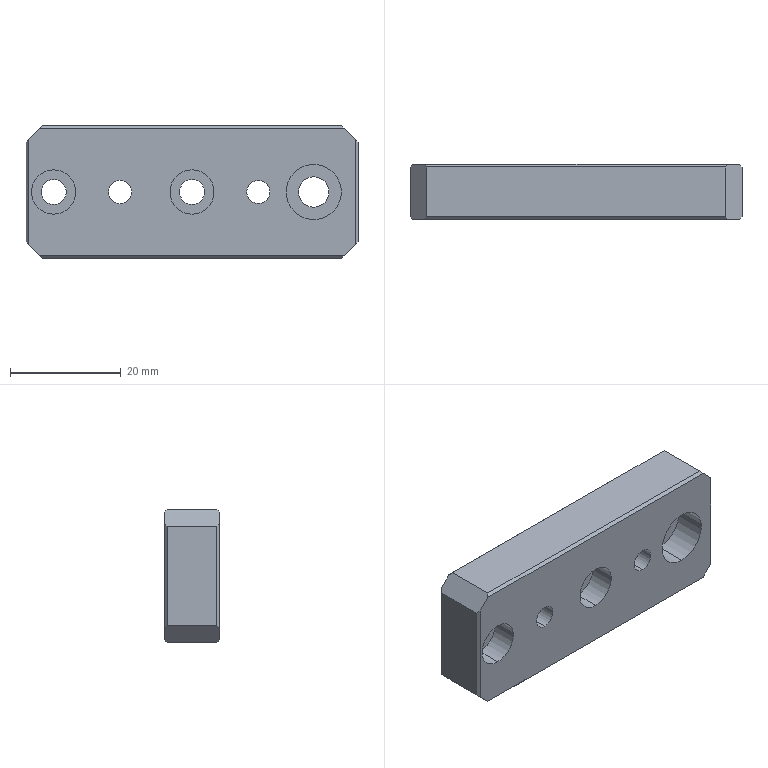Part | SolidWorks | features HoleWzd 4, Chamfer 2, Extrusion 1, ICE 1 | 1 solid | 37 faces | box 60 x 10 x 24 mm | volume 12723 mm3 | plane 21 | cylinder 16 | commonest cylinder face diameters 4.2 x4 4.5 x4 8 x4 5.5 x2 10 x2
STEP:
#1=CARTESIAN_POINT('',(-11.927,0.,1.064));
#2=VERTEX_POINT('',#1);
#3=CARTESIAN_POINT('',(-11.927,0.,5.264));
#4=VERTEX_POINT('',#3);
#5=CARTESIAN_POINT('',(-11.927,0.,3.164));
#6=DIRECTION('',(0.,1.,0.));
#7=DIRECTION('',(0.,0.,1.));
#8=AXIS2_PLACEMENT_3D('',#5,#6,#7);
#9=CIRCLE('',#8,2.1);
#10=EDGE_CURVE('',#2,#4,#9,.T.);
#11=ORIENTED_EDGE('',*,*,#10,.F.);
#12=CARTESIAN_POINT('',(-11.927,10.,1.064));
#13=VERTEX_POINT('',#12);
#14=CARTESIAN_POINT('',(-11.927,10.,1.064));
#15=DIRECTION('',(0.,1.,0.));
#16=VECTOR('',#15,1000.);
#17=LINE('',#14,#16);
#18=EDGE_CURVE('',#2,#13,#17,.T.);
#19=ORIENTED_EDGE('',*,*,#18,.T.);
#20=CARTESIAN_POINT('',(-11.927,10.,5.264));
#21=VERTEX_POINT('',#20);
#22=CARTESIAN_POINT('',(-11.927,10.,3.164));
#23=DIRECTION('',(0.,1.,0.));
#24=DIRECTION('',(0.,0.,1.));
#25=AXIS2_PLACEMENT_3D('',#22,#23,#24);
#26=CIRCLE('',#25,2.1);
#27=EDGE_CURVE('',#13,#21,#26,.T.);
#28=ORIENTED_EDGE('',*,*,#27,.T.);
#29=CARTESIAN_POINT('',(-11.927,10.,5.264));
#30=DIRECTION('',(0.,1.,0.));
#31=VECTOR('',#30,1000.);
#32=LINE('',#29,#31);
#33=EDGE_CURVE('',#4,#21,#32,.T.);
#34=ORIENTED_EDGE('',*,*,#33,.F.);
#35=EDGE_LOOP('',(#11,#19,#28,#34));
#36=FACE_OUTER_BOUND('',#35,.T.);
#37=CARTESIAN_POINT('',(-11.927,10.,3.164));
#38=DIRECTION('',(0.,1.,0.));
#39=DIRECTION('',(0.,0.,1.));
#40=AXIS2_PLACEMENT_3D('',#37,#38,#39);
#41=CYLINDRICAL_SURFACE('',#40,2.1);
#42=ADVANCED_FACE('',(#36),#41,.F.);
#43=CARTESIAN_POINT('',(13.073,0.,1.064));
#44=VERTEX_POINT('',#43);
#45=CARTESIAN_POINT('',(13.073,0.,5.264));
#46=VERTEX_POINT('',#45);
#47=CARTESIAN_POINT('',(13.073,0.,3.164));
#48=DIRECTION('',(0.,1.,0.));
#49=DIRECTION('',(0.,0.,1.));
#50=AXIS2_PLACEMENT_3D('',#47,#48,#49);
#51=CIRCLE('',#50,2.1);
#52=EDGE_CURVE('',#44,#46,#51,.T.);
#53=ORIENTED_EDGE('',*,*,#52,.F.);
#54=CARTESIAN_POINT('',(13.073,10.,1.064));
#55=VERTEX_POINT('',#54);
#56=CARTESIAN_POINT('',(13.073,10.,1.064));
#57=DIRECTION('',(0.,1.,0.));
#58=VECTOR('',#57,1000.);
#59=LINE('',#56,#58);
#60=EDGE_CURVE('',#44,#55,#59,.T.);
#61=ORIENTED_EDGE('',*,*,#60,.T.);
#62=CARTESIAN_POINT('',(13.073,10.,5.264));
#63=VERTEX_POINT('',#62);
#64=CARTESIAN_POINT('',(13.073,10.,3.164));
#65=DIRECTION('',(0.,1.,0.));
#66=DIRECTION('',(0.,0.,1.));
#67=AXIS2_PLACEMENT_3D('',#64,#65,#66);
#68=CIRCLE('',#67,2.1);
#69=EDGE_CURVE('',#55,#63,#68,.T.);
#70=ORIENTED_EDGE('',*,*,#69,.T.);
#71=CARTESIAN_POINT('',(13.073,10.,5.264));
#72=DIRECTION('',(0.,1.,0.));
#73=VECTOR('',#72,1000.);
#74=LINE('',#71,#73);
#75=EDGE_CURVE('',#46,#63,#74,.T.);
#76=ORIENTED_EDGE('',*,*,#75,.F.);
#77=EDGE_LOOP('',(#53,#61,#70,#76));
#78=FACE_OUTER_BOUND('',#77,.T.);
#79=CARTESIAN_POINT('',(13.073,10.,3.164));
#80=DIRECTION('',(0.,1.,0.));
#81=DIRECTION('',(0.,0.,1.));
#82=AXIS2_PLACEMENT_3D('',#79,#80,#81);
#83=CYLINDRICAL_SURFACE('',#82,2.1);
#84=ADVANCED_FACE('',(#78),#83,.F.);
#85=CARTESIAN_POINT('',(23.073,5.7,8.164));
#86=VERTEX_POINT('',#85);
#87=CARTESIAN_POINT('',(23.073,5.7,-1.836));
#88=VERTEX_POINT('',#87);
#89=CARTESIAN_POINT('',(23.073,5.7,3.164));
#90=DIRECTION('',(0.,-1.,0.));
#91=DIRECTION('',(0.,0.,-1.));
#92=AXIS2_PLACEMENT_3D('',#89,#90,#91);
#93=CIRCLE('',#92,5.);
#94=EDGE_CURVE('',#86,#88,#93,.T.);
#95=ORIENTED_EDGE('',*,*,#94,.F.);
#96=CARTESIAN_POINT('',(23.073,0.,8.164));
#97=VERTEX_POINT('',#96);
#98=CARTESIAN_POINT('',(23.073,0.,8.164));
#99=DIRECTION('',(0.,-1.,0.));
#100=VECTOR('',#99,1000.);
#101=LINE('',#98,#100);
#102=EDGE_CURVE('',#86,#97,#101,.T.);
#103=ORIENTED_EDGE('',*,*,#102,.T.);
#104=CARTESIAN_POINT('',(23.073,0.,-1.836));
#105=VERTEX_POINT('',#104);
#106=CARTESIAN_POINT('',(23.073,0.,3.164));
#107=DIRECTION('',(0.,-1.,0.));
#108=DIRECTION('',(0.,0.,-1.));
#109=AXIS2_PLACEMENT_3D('',#106,#107,#108);
#110=CIRCLE('',#109,5.);
#111=EDGE_CURVE('',#97,#105,#110,.T.);
#112=ORIENTED_EDGE('',*,*,#111,.T.);
#113=CARTESIAN_POINT('',(23.073,0.,-1.836));
#114=DIRECTION('',(0.,-1.,0.));
#115=VECTOR('',#114,1000.);
#116=LINE('',#113,#115);
#117=EDGE_CURVE('',#88,#105,#116,.T.);
#118=ORIENTED_EDGE('',*,*,#117,.F.);
#119=EDGE_LOOP('',(#95,#103,#112,#118));
#120=FACE_OUTER_BOUND('',#119,.T.);
#121=CARTESIAN_POINT('',(23.073,0.,3.164));
#122=DIRECTION('',(0.,-1.,0.));
#123=DIRECTION('',(0.,0.,-1.));
#124=AXIS2_PLACEMENT_3D('',#121,#122,#123);
#125=CYLINDRICAL_SURFACE('',#124,5.);
#126=ADVANCED_FACE('',(#120),#125,.F.);
#127=CARTESIAN_POINT('',(23.073,10.,0.4137));
#128=VERTEX_POINT('',#127);
#129=CARTESIAN_POINT('',(23.073,10.,5.914));
#130=VERTEX_POINT('',#129);
#131=CARTESIAN_POINT('',(23.073,10.,3.164));
#132=DIRECTION('',(0.,1.,0.));
#133=DIRECTION('',(0.,0.,1.));
#134=AXIS2_PLACEMENT_3D('',#131,#132,#133);
#135=CIRCLE('',#134,2.75);
#136=EDGE_CURVE('',#128,#130,#135,.T.);
#137=ORIENTED_EDGE('',*,*,#136,.T.);
#138=CARTESIAN_POINT('',(23.073,5.7,5.914));
#139=VERTEX_POINT('',#138);
#140=CARTESIAN_POINT('',(23.073,0.,5.914));
#141=DIRECTION('',(0.,-1.,0.));
#142=VECTOR('',#141,1000.);
#143=LINE('',#140,#142);
#144=EDGE_CURVE('',#130,#139,#143,.T.);
#145=ORIENTED_EDGE('',*,*,#144,.T.);
#146=CARTESIAN_POINT('',(23.073,5.7,0.4137));
#147=VERTEX_POINT('',#146);
#148=CARTESIAN_POINT('',(23.073,5.7,3.164));
#149=DIRECTION('',(0.,-1.,0.));
#150=DIRECTION('',(0.,0.,-1.));
#151=AXIS2_PLACEMENT_3D('',#148,#149,#150);
#152=CIRCLE('',#151,2.75);
#153=EDGE_CURVE('',#139,#147,#152,.T.);
#154=ORIENTED_EDGE('',*,*,#153,.T.);
#155=CARTESIAN_POINT('',(23.073,0.,0.4137));
#156=DIRECTION('',(0.,-1.,0.));
#157=VECTOR('',#156,1000.);
#158=LINE('',#155,#157);
#159=EDGE_CURVE('',#128,#147,#158,.T.);
#160=ORIENTED_EDGE('',*,*,#159,.F.);
#161=EDGE_LOOP('',(#137,#145,#154,#160));
#162=FACE_OUTER_BOUND('',#161,.T.);
#163=CARTESIAN_POINT('',(23.073,0.,3.164));
#164=DIRECTION('',(0.,-1.,0.));
#165=DIRECTION('',(0.,0.,-1.));
#166=AXIS2_PLACEMENT_3D('',#163,#164,#165);
#167=CYLINDRICAL_SURFACE('',#166,2.75);
#168=ADVANCED_FACE('',(#162),#167,.F.);
#169=CARTESIAN_POINT('',(-23.927,4.6,7.164));
#170=VERTEX_POINT('',#169);
#171=CARTESIAN_POINT('',(-23.927,4.6,-0.8363));
#172=VERTEX_POINT('',#171);
#173=CARTESIAN_POINT('',(-23.927,4.6,3.164));
#174=DIRECTION('',(0.,-1.,0.));
#175=DIRECTION('',(0.,0.,-1.));
#176=AXIS2_PLACEMENT_3D('',#173,#174,#175);
#177=CIRCLE('',#176,4.);
#178=EDGE_CURVE('',#170,#172,#177,.T.);
#179=ORIENTED_EDGE('',*,*,#178,.F.);
#180=CARTESIAN_POINT('',(-23.927,0.,7.164));
#181=VERTEX_POINT('',#180);
#182=CARTESIAN_POINT('',(-23.927,0.,7.164));
#183=DIRECTION('',(0.,-1.,0.));
#184=VECTOR('',#183,1000.);
#185=LINE('',#182,#184);
#186=EDGE_CURVE('',#170,#181,#185,.T.);
#187=ORIENTED_EDGE('',*,*,#186,.T.);
#188=CARTESIAN_POINT('',(-23.927,0.,-0.8363));
#189=VERTEX_POINT('',#188);
#190=CARTESIAN_POINT('',(-23.927,0.,3.164));
#191=DIRECTION('',(0.,-1.,0.));
#192=DIRECTION('',(0.,0.,-1.));
#193=AXIS2_PLACEMENT_3D('',#190,#191,#192);
#194=CIRCLE('',#193,4.);
#195=EDGE_CURVE('',#181,#189,#194,.T.);
#196=ORIENTED_EDGE('',*,*,#195,.T.);
#197=CARTESIAN_POINT('',(-23.927,0.,-0.8363));
#198=DIRECTION('',(0.,-1.,0.));
#199=VECTOR('',#198,1000.);
#200=LINE('',#197,#199);
#201=EDGE_CURVE('',#172,#189,#200,.T.);
#202=ORIENTED_EDGE('',*,*,#201,.F.);
#203=EDGE_LOOP('',(#179,#187,#196,#202));
#204=FACE_OUTER_BOUND('',#203,.T.);
#205=CARTESIAN_POINT('',(-23.927,0.,3.164));
#206=DIRECTION('',(0.,-1.,0.));
#207=DIRECTION('',(0.,0.,-1.));
#208=AXIS2_PLACEMENT_3D('',#205,#206,#207);
#209=CYLINDRICAL_SURFACE('',#208,4.);
#210=ADVANCED_FACE('',(#204),#209,.F.);
#211=CARTESIAN_POINT('',(-23.927,10.,0.9137));
#212=VERTEX_POINT('',#211);
#213=CARTESIAN_POINT('',(-23.927,10.,5.414));
#214=VERTEX_POINT('',#213);
#215=CARTESIAN_POINT('',(-23.927,10.,3.164));
#216=DIRECTION('',(0.,1.,0.));
#217=DIRECTION('',(0.,0.,1.));
#218=AXIS2_PLACEMENT_3D('',#215,#216,#217);
#219=CIRCLE('',#218,2.25);
#220=EDGE_CURVE('',#212,#214,#219,.T.);
#221=ORIENTED_EDGE('',*,*,#220,.T.);
#222=CARTESIAN_POINT('',(-23.927,4.6,5.414));
#223=VERTEX_POINT('',#222);
#224=CARTESIAN_POINT('',(-23.927,0.,5.414));
#225=DIRECTION('',(0.,-1.,0.));
#226=VECTOR('',#225,1000.);
#227=LINE('',#224,#226);
#228=EDGE_CURVE('',#214,#223,#227,.T.);
#229=ORIENTED_EDGE('',*,*,#228,.T.);
#230=CARTESIAN_POINT('',(-23.927,4.6,0.9137));
#231=VERTEX_POINT('',#230);
#232=CARTESIAN_POINT('',(-23.927,4.6,3.164));
#233=DIRECTION('',(0.,-1.,0.));
#234=DIRECTION('',(0.,0.,-1.));
#235=AXIS2_PLACEMENT_3D('',#232,#233,#234);
#236=CIRCLE('',#235,2.25);
#237=EDGE_CURVE('',#223,#231,#236,.T.);
#238=ORIENTED_EDGE('',*,*,#237,.T.);
#239=CARTESIAN_POINT('',(-23.927,0.,0.9137));
#240=DIRECTION('',(0.,-1.,0.));
#241=VECTOR('',#240,1000.);
#242=LINE('',#239,#241);
#243=EDGE_CURVE('',#212,#231,#242,.T.);
#244=ORIENTED_EDGE('',*,*,#243,.F.);
#245=EDGE_LOOP('',(#221,#229,#238,#244));
#246=FACE_OUTER_BOUND('',#245,.T.);
#247=CARTESIAN_POINT('',(-23.927,0.,3.164));
#248=DIRECTION('',(0.,-1.,0.));
#249=DIRECTION('',(0.,0.,-1.));
#250=AXIS2_PLACEMENT_3D('',#247,#248,#249);
#251=CYLINDRICAL_SURFACE('',#250,2.25);
#252=ADVANCED_FACE('',(#246),#251,.F.);
#253=CARTESIAN_POINT('',(1.073,4.6,7.164));
#254=VERTEX_POINT('',#253);
#255=CARTESIAN_POINT('',(1.073,4.6,-0.8363));
#256=VERTEX_POINT('',#255);
#257=CARTESIAN_POINT('',(1.073,4.6,3.164));
#258=DIRECTION('',(0.,-1.,0.));
#259=DIRECTION('',(0.,0.,-1.));
#260=AXIS2_PLACEMENT_3D('',#257,#258,#259);
#261=CIRCLE('',#260,4.);
#262=EDGE_CURVE('',#254,#256,#261,.T.);
#263=ORIENTED_EDGE('',*,*,#262,.F.);
#264=CARTESIAN_POINT('',(1.073,0.,7.164));
#265=VERTEX_POINT('',#264);
#266=CARTESIAN_POINT('',(1.073,0.,7.164));
#267=DIRECTION('',(0.,-1.,0.));
#268=VECTOR('',#267,1000.);
#269=LINE('',#266,#268);
#270=EDGE_CURVE('',#254,#265,#269,.T.);
#271=ORIENTED_EDGE('',*,*,#270,.T.);
#272=CARTESIAN_POINT('',(1.073,0.,-0.8363));
#273=VERTEX_POINT('',#272);
#274=CARTESIAN_POINT('',(1.073,0.,3.164));
#275=DIRECTION('',(0.,-1.,0.));
#276=DIRECTION('',(0.,0.,-1.));
#277=AXIS2_PLACEMENT_3D('',#274,#275,#276);
#278=CIRCLE('',#277,4.);
#279=EDGE_CURVE('',#265,#273,#278,.T.);
#280=ORIENTED_EDGE('',*,*,#279,.T.);
#281=CARTESIAN_POINT('',(1.073,0.,-0.8363));
#282=DIRECTION('',(0.,-1.,0.));
#283=VECTOR('',#282,1000.);
#284=LINE('',#281,#283);
#285=EDGE_CURVE('',#256,#273,#284,.T.);
#286=ORIENTED_EDGE('',*,*,#285,.F.);
#287=EDGE_LOOP('',(#263,#271,#280,#286));
#288=FACE_OUTER_BOUND('',#287,.T.);
#289=CARTESIAN_POINT('',(1.073,0.,3.164));
#290=DIRECTION('',(0.,-1.,0.));
#291=DIRECTION('',(0.,0.,-1.));
#292=AXIS2_PLACEMENT_3D('',#289,#290,#291);
#293=CYLINDRICAL_SURFACE('',#292,4.);
#294=ADVANCED_FACE('',(#288),#293,.F.);
#295=CARTESIAN_POINT('',(1.073,10.,0.9137));
#296=VERTEX_POINT('',#295);
#297=CARTESIAN_POINT('',(1.073,10.,5.414));
#298=VERTEX_POINT('',#297);
#299=CARTESIAN_POINT('',(1.073,10.,3.164));
#300=DIRECTION('',(0.,1.,0.));
#301=DIRECTION('',(0.,0.,1.));
#302=AXIS2_PLACEMENT_3D('',#299,#300,#301);
#303=CIRCLE('',#302,2.25);
#304=EDGE_CURVE('',#296,#298,#303,.T.);
#305=ORIENTED_EDGE('',*,*,#304,.T.);
#306=CARTESIAN_POINT('',(1.073,4.6,5.414));
#307=VERTEX_POINT('',#306);
#308=CARTESIAN_POINT('',(1.073,0.,5.414));
#309=DIRECTION('',(0.,-1.,0.));
#310=VECTOR('',#309,1000.);
#311=LINE('',#308,#310);
#312=EDGE_CURVE('',#298,#307,#311,.T.);
#313=ORIENTED_EDGE('',*,*,#312,.T.);
#314=CARTESIAN_POINT('',(1.073,4.6,0.9137));
#315=VERTEX_POINT('',#314);
#316=CARTESIAN_POINT('',(1.073,4.6,3.164));
#317=DIRECTION('',(0.,-1.,0.));
#318=DIRECTION('',(0.,0.,-1.));
#319=AXIS2_PLACEMENT_3D('',#316,#317,#318);
#320=CIRCLE('',#319,2.25);
#321=EDGE_CURVE('',#307,#315,#320,.T.);
#322=ORIENTED_EDGE('',*,*,#321,.T.);
#323=CARTESIAN_POINT('',(1.073,0.,0.9137));
#324=DIRECTION('',(0.,-1.,0.));
#325=VECTOR('',#324,1000.);
#326=LINE('',#323,#325);
#327=EDGE_CURVE('',#296,#315,#326,.T.);
#328=ORIENTED_EDGE('',*,*,#327,.F.);
#329=EDGE_LOOP('',(#305,#313,#322,#328));
#330=FACE_OUTER_BOUND('',#329,.T.);
#331=CARTESIAN_POINT('',(1.073,0.,3.164));
#332=DIRECTION('',(0.,-1.,0.));
#333=DIRECTION('',(0.,0.,-1.));
#334=AXIS2_PLACEMENT_3D('',#331,#332,#333);
#335=CYLINDRICAL_SURFACE('',#334,2.25);
#336=ADVANCED_FACE('',(#330),#335,.F.);
#337=CARTESIAN_POINT('',(-28.927,9.5,-5.836));
#338=VERTEX_POINT('',#337);
#339=CARTESIAN_POINT('',(-28.927,0.5,-5.836));
#340=VERTEX_POINT('',#339);
#341=CARTESIAN_POINT('',(-28.927,10.,-5.836));
#342=DIRECTION('',(0.,-1.,0.));
#343=VECTOR('',#342,1000.);
#344=LINE('',#341,#343);
#345=EDGE_CURVE('',#338,#340,#344,.T.);
#346=ORIENTED_EDGE('',*,*,#345,.T.);
#347=CARTESIAN_POINT('',(-28.927,0.5,12.164));
#348=VERTEX_POINT('',#347);
#349=CARTESIAN_POINT('',(-28.927,0.5,-8.836));
#350=DIRECTION('',(0.,0.,1.));
#351=VECTOR('',#350,1000.);
#352=LINE('',#349,#351);
#353=EDGE_CURVE('',#340,#348,#352,.T.);
#354=ORIENTED_EDGE('',*,*,#353,.T.);
#355=CARTESIAN_POINT('',(-28.927,9.5,12.164));
#356=VERTEX_POINT('',#355);
#357=CARTESIAN_POINT('',(-28.927,10.,12.164));
#358=DIRECTION('',(0.,1.,0.));
#359=VECTOR('',#358,1000.);
#360=LINE('',#357,#359);
#361=EDGE_CURVE('',#348,#356,#360,.T.);
#362=ORIENTED_EDGE('',*,*,#361,.T.);
#363=CARTESIAN_POINT('',(-28.927,9.5,-5.836));
#364=DIRECTION('',(0.,0.,-1.));
#365=VECTOR('',#364,1000.);
#366=LINE('',#363,#365);
#367=EDGE_CURVE('',#356,#338,#366,.T.);
#368=ORIENTED_EDGE('',*,*,#367,.T.);
#369=EDGE_LOOP('',(#346,#354,#362,#368));
#370=FACE_OUTER_BOUND('',#369,.T.);
#371=CARTESIAN_POINT('',(-28.927,10.,-8.836));
#372=DIRECTION('',(1.,0.,0.));
#373=DIRECTION('',(0.,0.,-1.));
#374=AXIS2_PLACEMENT_3D('',#371,#372,#373);
#375=PLANE('',#374);
#376=ADVANCED_FACE('',(#370),#375,.F.);
#377=CARTESIAN_POINT('',(-25.927,9.5,15.164));
#378=VERTEX_POINT('',#377);
#379=CARTESIAN_POINT('',(-25.927,0.5,15.164));
#380=VERTEX_POINT('',#379);
#381=CARTESIAN_POINT('',(-25.927,10.,15.164));
#382=DIRECTION('',(0.,-1.,0.));
#383=VECTOR('',#382,1000.);
#384=LINE('',#381,#383);
#385=EDGE_CURVE('',#378,#380,#384,.T.);
#386=ORIENTED_EDGE('',*,*,#385,.T.);
#387=CARTESIAN_POINT('',(28.073,0.5,15.164));
#388=VERTEX_POINT('',#387);
#389=CARTESIAN_POINT('',(-28.927,0.5,15.164));
#390=DIRECTION('',(1.,0.,0.));
#391=VECTOR('',#390,1000.);
#392=LINE('',#389,#391);
#393=EDGE_CURVE('',#380,#388,#392,.T.);
#394=ORIENTED_EDGE('',*,*,#393,.T.);
#395=CARTESIAN_POINT('',(28.073,9.5,15.164));
#396=VERTEX_POINT('',#395);
#397=CARTESIAN_POINT('',(28.073,10.,15.164));
#398=DIRECTION('',(0.,1.,0.));
#399=VECTOR('',#398,1000.);
#400=LINE('',#397,#399);
#401=EDGE_CURVE('',#388,#396,#400,.T.);
#402=ORIENTED_EDGE('',*,*,#401,.T.);
#403=CARTESIAN_POINT('',(-25.927,9.5,15.164));
#404=DIRECTION('',(-1.,0.,0.));
#405=VECTOR('',#404,1000.);
#406=LINE('',#403,#405);
#407=EDGE_CURVE('',#396,#378,#406,.T.);
#408=ORIENTED_EDGE('',*,*,#407,.T.);
#409=EDGE_LOOP('',(#386,#394,#402,#408));
#410=FACE_OUTER_BOUND('',#409,.T.);
#411=CARTESIAN_POINT('',(-28.927,10.,15.164));
#412=DIRECTION('',(0.,0.,-1.));
#413=DIRECTION('',(-1.,0.,0.));
#414=AXIS2_PLACEMENT_3D('',#411,#412,#413);
#415=PLANE('',#414);
#416=ADVANCED_FACE('',(#410),#415,.F.);
#417=CARTESIAN_POINT('',(28.073,9.5,-8.836));
#418=VERTEX_POINT('',#417);
#419=CARTESIAN_POINT('',(28.073,0.5,-8.836));
#420=VERTEX_POINT('',#419);
#421=CARTESIAN_POINT('',(28.073,10.,-8.836));
#422=DIRECTION('',(0.,-1.,0.));
#423=VECTOR('',#422,1000.);
#424=LINE('',#421,#423);
#425=EDGE_CURVE('',#418,#420,#424,.T.);
#426=ORIENTED_EDGE('',*,*,#425,.T.);
#427=CARTESIAN_POINT('',(-25.927,0.5,-8.836));
#428=VERTEX_POINT('',#427);
#429=CARTESIAN_POINT('',(-28.927,0.5,-8.836));
#430=DIRECTION('',(-1.,0.,0.));
#431=VECTOR('',#430,1000.);
#432=LINE('',#429,#431);
#433=EDGE_CURVE('',#420,#428,#432,.T.);
#434=ORIENTED_EDGE('',*,*,#433,.T.);
#435=CARTESIAN_POINT('',(-25.927,9.5,-8.836));
#436=VERTEX_POINT('',#435);
#437=CARTESIAN_POINT('',(-25.927,10.,-8.836));
#438=DIRECTION('',(0.,1.,0.));
#439=VECTOR('',#438,1000.);
#440=LINE('',#437,#439);
#441=EDGE_CURVE('',#428,#436,#440,.T.);
#442=ORIENTED_EDGE('',*,*,#441,.T.);
#443=CARTESIAN_POINT('',(28.073,9.5,-8.836));
#444=DIRECTION('',(1.,0.,0.));
#445=VECTOR('',#444,1000.);
#446=LINE('',#443,#445);
#447=EDGE_CURVE('',#436,#418,#446,.T.);
#448=ORIENTED_EDGE('',*,*,#447,.T.);
#449=EDGE_LOOP('',(#426,#434,#442,#448));
#450=FACE_OUTER_BOUND('',#449,.T.);
#451=CARTESIAN_POINT('',(-28.927,10.,-8.836));
#452=DIRECTION('',(0.,0.,1.));
#453=DIRECTION('',(1.,0.,0.));
#454=AXIS2_PLACEMENT_3D('',#451,#452,#453);
#455=PLANE('',#454);
#456=ADVANCED_FACE('',(#450),#455,.F.);
#457=CARTESIAN_POINT('',(-11.927,10.,3.164));
#458=DIRECTION('',(0.,1.,0.));
#459=DIRECTION('',(0.,0.,1.));
#460=AXIS2_PLACEMENT_3D('',#457,#458,#459);
#461=CIRCLE('',#460,2.1);
#462=EDGE_CURVE('',#21,#13,#461,.T.);
#463=ORIENTED_EDGE('',*,*,#462,.F.);
#464=ORIENTED_EDGE('',*,*,#27,.F.);
#465=EDGE_LOOP('',(#463,#464));
#466=FACE_BOUND('',#465,.T.);
#467=CARTESIAN_POINT('',(13.073,10.,3.164));
#468=DIRECTION('',(0.,1.,0.));
#469=DIRECTION('',(0.,0.,1.));
#470=AXIS2_PLACEMENT_3D('',#467,#468,#469);
#471=CIRCLE('',#470,2.1);
#472=EDGE_CURVE('',#63,#55,#471,.T.);
#473=ORIENTED_EDGE('',*,*,#472,.F.);
#474=ORIENTED_EDGE('',*,*,#69,.F.);
#475=EDGE_LOOP('',(#473,#474));
#476=FACE_BOUND('',#475,.T.);
#477=ORIENTED_EDGE('',*,*,#136,.F.);
#478=CARTESIAN_POINT('',(23.073,10.,3.164));
#479=DIRECTION('',(0.,1.,0.));
#480=DIRECTION('',(0.,0.,1.));
#481=AXIS2_PLACEMENT_3D('',#478,#479,#480);
#482=CIRCLE('',#481,2.75);
#483=EDGE_CURVE('',#130,#128,#482,.T.);
#484=ORIENTED_EDGE('',*,*,#483,.F.);
#485=EDGE_LOOP('',(#477,#484));
#486=FACE_BOUND('',#485,.T.);
#487=ORIENTED_EDGE('',*,*,#220,.F.);
#488=CARTESIAN_POINT('',(-23.927,10.,3.164));
#489=DIRECTION('',(0.,1.,0.));
#490=DIRECTION('',(0.,0.,1.));
#491=AXIS2_PLACEMENT_3D('',#488,#489,#490);
#492=CIRCLE('',#491,2.25);
#493=EDGE_CURVE('',#214,#212,#492,.T.);
#494=ORIENTED_EDGE('',*,*,#493,.F.);
#495=EDGE_LOOP('',(#487,#494));
#496=FACE_BOUND('',#495,.T.);
#497=ORIENTED_EDGE('',*,*,#304,.F.);
#498=CARTESIAN_POINT('',(1.073,10.,3.164));
#499=DIRECTION('',(0.,1.,0.));
#500=DIRECTION('',(0.,0.,1.));
#501=AXIS2_PLACEMENT_3D('',#498,#499,#500);
#502=CIRCLE('',#501,2.25);
#503=EDGE_CURVE('',#298,#296,#502,.T.);
#504=ORIENTED_EDGE('',*,*,#503,.F.);
#505=EDGE_LOOP('',(#497,#504));
#506=FACE_BOUND('',#505,.T.);
#507=CARTESIAN_POINT('',(28.573,10.,14.664));
#508=VERTEX_POINT('',#507);
#509=CARTESIAN_POINT('',(30.573,10.,12.664));
#510=VERTEX_POINT('',#509);
#511=CARTESIAN_POINT('',(-0.4271,10.,43.664));
#512=DIRECTION('',(0.7071,0.,-0.7071));
#513=VECTOR('',#512,1000.);
#514=LINE('',#511,#513);
#515=EDGE_CURVE('',#508,#510,#514,.T.);
#516=ORIENTED_EDGE('',*,*,#515,.T.);
#517=CARTESIAN_POINT('',(30.573,10.,-6.336));
#518=VERTEX_POINT('',#517);
#519=CARTESIAN_POINT('',(30.573,10.,-5.836));
#520=DIRECTION('',(0.,0.,-1.));
#521=VECTOR('',#520,1000.);
#522=LINE('',#519,#521);
#523=EDGE_CURVE('',#510,#518,#522,.T.);
#524=ORIENTED_EDGE('',*,*,#523,.T.);
#525=CARTESIAN_POINT('',(28.573,10.,-8.336));
#526=VERTEX_POINT('',#525);
#527=CARTESIAN_POINT('',(11.573,10.,-25.336));
#528=DIRECTION('',(-0.7071,0.,-0.7071));
#529=VECTOR('',#528,1000.);
#530=LINE('',#527,#529);
#531=EDGE_CURVE('',#518,#526,#530,.T.);
#532=ORIENTED_EDGE('',*,*,#531,.T.);
#533=CARTESIAN_POINT('',(-26.427,10.,-8.336));
#534=VERTEX_POINT('',#533);
#535=CARTESIAN_POINT('',(-25.927,10.,-8.336));
#536=DIRECTION('',(-1.,0.,0.));
#537=VECTOR('',#536,1000.);
#538=LINE('',#535,#537);
#539=EDGE_CURVE('',#526,#534,#538,.T.);
#540=ORIENTED_EDGE('',*,*,#539,.T.);
#541=CARTESIAN_POINT('',(-28.427,10.,-6.336));
#542=VERTEX_POINT('',#541);
#543=CARTESIAN_POINT('',(-39.427,10.,4.664));
#544=DIRECTION('',(-0.7071,0.,0.7071));
#545=VECTOR('',#544,1000.);
#546=LINE('',#543,#545);
#547=EDGE_CURVE('',#534,#542,#546,.T.);
#548=ORIENTED_EDGE('',*,*,#547,.T.);
#549=CARTESIAN_POINT('',(-28.427,10.,12.664));
#550=VERTEX_POINT('',#549);
#551=CARTESIAN_POINT('',(-28.427,10.,12.164));
#552=DIRECTION('',(0.,0.,1.));
#553=VECTOR('',#552,1000.);
#554=LINE('',#551,#553);
#555=EDGE_CURVE('',#542,#550,#554,.T.);
#556=ORIENTED_EDGE('',*,*,#555,.T.);
#557=CARTESIAN_POINT('',(-26.427,10.,14.664));
#558=VERTEX_POINT('',#557);
#559=CARTESIAN_POINT('',(-27.427,10.,13.664));
#560=DIRECTION('',(0.7071,0.,0.7071));
#561=VECTOR('',#560,1000.);
#562=LINE('',#559,#561);
#563=EDGE_CURVE('',#550,#558,#562,.T.);
#564=ORIENTED_EDGE('',*,*,#563,.T.);
#565=CARTESIAN_POINT('',(28.073,10.,14.664));
#566=DIRECTION('',(1.,0.,0.));
#567=VECTOR('',#566,1000.);
#568=LINE('',#565,#567);
#569=EDGE_CURVE('',#558,#508,#568,.T.);
#570=ORIENTED_EDGE('',*,*,#569,.T.);
#571=EDGE_LOOP('',(#516,#524,#532,#540,#548,#556,#564,#570));
#572=FACE_OUTER_BOUND('',#571,.T.);
#573=CARTESIAN_POINT('',(-28.927,10.,15.164));
#574=DIRECTION('',(0.,1.,0.));
#575=DIRECTION('',(0.,0.,1.));
#576=AXIS2_PLACEMENT_3D('',#573,#574,#575);
#577=PLANE('',#576);
#578=ADVANCED_FACE('',(#466,#476,#486,#496,#506,#572),#577,.T.);
#579=CARTESIAN_POINT('',(-11.927,0.,3.164));
#580=DIRECTION('',(0.,1.,0.));
#581=DIRECTION('',(0.,0.,1.));
#582=AXIS2_PLACEMENT_3D('',#579,#580,#581);
#583=CIRCLE('',#582,2.1);
#584=EDGE_CURVE('',#4,#2,#583,.T.);
#585=ORIENTED_EDGE('',*,*,#584,.T.);
#586=ORIENTED_EDGE('',*,*,#10,.T.);
#587=EDGE_LOOP('',(#585,#586));
#588=FACE_BOUND('',#587,.T.);
#589=CARTESIAN_POINT('',(13.073,0.,3.164));
#590=DIRECTION('',(0.,1.,0.));
#591=DIRECTION('',(0.,0.,1.));
#592=AXIS2_PLACEMENT_3D('',#589,#590,#591);
#593=CIRCLE('',#592,2.1);
#594=EDGE_CURVE('',#46,#44,#593,.T.);
#595=ORIENTED_EDGE('',*,*,#594,.T.);
#596=ORIENTED_EDGE('',*,*,#52,.T.);
#597=EDGE_LOOP('',(#595,#596));
#598=FACE_BOUND('',#597,.T.);
#599=CARTESIAN_POINT('',(23.073,0.,3.164));
#600=DIRECTION('',(0.,-1.,0.));
#601=DIRECTION('',(0.,0.,-1.));
#602=AXIS2_PLACEMENT_3D('',#599,#600,#601);
#603=CIRCLE('',#602,5.);
#604=EDGE_CURVE('',#105,#97,#603,.T.);
#605=ORIENTED_EDGE('',*,*,#604,.F.);
#606=ORIENTED_EDGE('',*,*,#111,.F.);
#607=EDGE_LOOP('',(#605,#606));
#608=FACE_BOUND('',#607,.T.);
#609=CARTESIAN_POINT('',(-23.927,0.,3.164));
#610=DIRECTION('',(0.,-1.,0.));
#611=DIRECTION('',(0.,0.,-1.));
#612=AXIS2_PLACEMENT_3D('',#609,#610,#611);
#613=CIRCLE('',#612,4.);
#614=EDGE_CURVE('',#189,#181,#613,.T.);
#615=ORIENTED_EDGE('',*,*,#614,.F.);
#616=ORIENTED_EDGE('',*,*,#195,.F.);
#617=EDGE_LOOP('',(#615,#616));
#618=FACE_BOUND('',#617,.T.);
#619=CARTESIAN_POINT('',(1.073,0.,3.164));
#620=DIRECTION('',(0.,-1.,0.));
#621=DIRECTION('',(0.,0.,-1.));
#622=AXIS2_PLACEMENT_3D('',#619,#620,#621);
#623=CIRCLE('',#622,4.);
#624=EDGE_CURVE('',#273,#265,#623,.T.);
#625=ORIENTED_EDGE('',*,*,#624,.F.);
#626=ORIENTED_EDGE('',*,*,#279,.F.);
#627=EDGE_LOOP('',(#625,#626));
#628=FACE_BOUND('',#627,.T.);
#629=CARTESIAN_POINT('',(28.573,0.,-8.336));
#630=VERTEX_POINT('',#629);
#631=CARTESIAN_POINT('',(30.573,0.,-6.336));
#632=VERTEX_POINT('',#631);
#633=CARTESIAN_POINT('',(28.073,0.,-8.836));
#634=DIRECTION('',(0.7071,0.,0.7071));
#635=VECTOR('',#634,1000.);
#636=LINE('',#633,#635);
#637=EDGE_CURVE('',#630,#632,#636,.T.);
#638=ORIENTED_EDGE('',*,*,#637,.T.);
#639=CARTESIAN_POINT('',(30.573,0.,12.664));
#640=VERTEX_POINT('',#639);
#641=CARTESIAN_POINT('',(30.573,0.,15.164));
#642=DIRECTION('',(0.,0.,1.));
#643=VECTOR('',#642,1000.);
#644=LINE('',#641,#643);
#645=EDGE_CURVE('',#632,#640,#644,.T.);
#646=ORIENTED_EDGE('',*,*,#645,.T.);
#647=CARTESIAN_POINT('',(28.573,0.,14.664));
#648=VERTEX_POINT('',#647);
#649=CARTESIAN_POINT('',(31.073,0.,12.164));
#650=DIRECTION('',(-0.7071,0.,0.7071));
#651=VECTOR('',#650,1000.);
#652=LINE('',#649,#651);
#653=EDGE_CURVE('',#640,#648,#652,.T.);
#654=ORIENTED_EDGE('',*,*,#653,.T.);
#655=CARTESIAN_POINT('',(-26.427,0.,14.664));
#656=VERTEX_POINT('',#655);
#657=CARTESIAN_POINT('',(-28.927,0.,14.664));
#658=DIRECTION('',(-1.,0.,0.));
#659=VECTOR('',#658,1000.);
#660=LINE('',#657,#659);
#661=EDGE_CURVE('',#648,#656,#660,.T.);
#662=ORIENTED_EDGE('',*,*,#661,.T.);
#663=CARTESIAN_POINT('',(-28.427,0.,12.664));
#664=VERTEX_POINT('',#663);
#665=CARTESIAN_POINT('',(-25.927,0.,15.164));
#666=DIRECTION('',(-0.7071,0.,-0.7071));
#667=VECTOR('',#666,1000.);
#668=LINE('',#665,#667);
#669=EDGE_CURVE('',#656,#664,#668,.T.);
#670=ORIENTED_EDGE('',*,*,#669,.T.);
#671=CARTESIAN_POINT('',(-28.427,0.,-6.336));
#672=VERTEX_POINT('',#671);
#673=CARTESIAN_POINT('',(-28.427,0.,15.164));
#674=DIRECTION('',(0.,0.,-1.));
#675=VECTOR('',#674,1000.);
#676=LINE('',#673,#675);
#677=EDGE_CURVE('',#664,#672,#676,.T.);
#678=ORIENTED_EDGE('',*,*,#677,.T.);
#679=CARTESIAN_POINT('',(-26.427,0.,-8.336));
#680=VERTEX_POINT('',#679);
#681=CARTESIAN_POINT('',(-28.927,0.,-5.836));
#682=DIRECTION('',(0.7071,0.,-0.7071));
#683=VECTOR('',#682,1000.);
#684=LINE('',#681,#683);
#685=EDGE_CURVE('',#672,#680,#684,.T.);
#686=ORIENTED_EDGE('',*,*,#685,.T.);
#687=CARTESIAN_POINT('',(-28.927,0.,-8.336));
#688=DIRECTION('',(1.,0.,0.));
#689=VECTOR('',#688,1000.);
#690=LINE('',#687,#689);
#691=EDGE_CURVE('',#680,#630,#690,.T.);
#692=ORIENTED_EDGE('',*,*,#691,.T.);
#693=EDGE_LOOP('',(#638,#646,#654,#662,#670,#678,#686,#692));
#694=FACE_OUTER_BOUND('',#693,.T.);
#695=CARTESIAN_POINT('',(-28.927,0.,15.164));
#696=DIRECTION('',(0.,1.,0.));
#697=DIRECTION('',(0.,0.,1.));
#698=AXIS2_PLACEMENT_3D('',#695,#696,#697);
#699=PLANE('',#698);
#700=ADVANCED_FACE('',(#588,#598,#608,#618,#628,#694),#699,.F.);
#701=ORIENTED_EDGE('',*,*,#312,.F.);
#702=ORIENTED_EDGE('',*,*,#503,.T.);
#703=ORIENTED_EDGE('',*,*,#327,.T.);
#704=CARTESIAN_POINT('',(1.073,4.6,3.164));
#705=DIRECTION('',(0.,-1.,0.));
#706=DIRECTION('',(0.,0.,-1.));
#707=AXIS2_PLACEMENT_3D('',#704,#705,#706);
#708=CIRCLE('',#707,2.25);
#709=EDGE_CURVE('',#315,#307,#708,.T.);
#710=ORIENTED_EDGE('',*,*,#709,.T.);
#711=EDGE_LOOP('',(#701,#702,#703,#710));
#712=FACE_OUTER_BOUND('',#711,.T.);
#713=CARTESIAN_POINT('',(1.073,0.,3.164));
#714=DIRECTION('',(0.,-1.,0.));
#715=DIRECTION('',(0.,0.,-1.));
#716=AXIS2_PLACEMENT_3D('',#713,#714,#715);
#717=CYLINDRICAL_SURFACE('',#716,2.25);
#718=ADVANCED_FACE('',(#712),#717,.F.);
#719=ORIENTED_EDGE('',*,*,#709,.F.);
#720=ORIENTED_EDGE('',*,*,#321,.F.);
#721=EDGE_LOOP('',(#719,#720));
#722=FACE_BOUND('',#721,.T.);
#723=CARTESIAN_POINT('',(1.073,4.6,3.164));
#724=DIRECTION('',(0.,-1.,0.));
#725=DIRECTION('',(0.,0.,-1.));
#726=AXIS2_PLACEMENT_3D('',#723,#724,#725);
#727=CIRCLE('',#726,4.);
#728=EDGE_CURVE('',#256,#254,#727,.T.);
#729=ORIENTED_EDGE('',*,*,#728,.T.);
#730=ORIENTED_EDGE('',*,*,#262,.T.);
#731=EDGE_LOOP('',(#729,#730));
#732=FACE_OUTER_BOUND('',#731,.T.);
#733=CARTESIAN_POINT('',(3.323,4.6,3.164));
#734=DIRECTION('',(0.,1.,0.));
#735=DIRECTION('',(0.,0.,1.));
#736=AXIS2_PLACEMENT_3D('',#733,#734,#735);
#737=PLANE('',#736);
#738=ADVANCED_FACE('',(#722,#732),#737,.F.);
#739=ORIENTED_EDGE('',*,*,#270,.F.);
#740=ORIENTED_EDGE('',*,*,#728,.F.);
#741=ORIENTED_EDGE('',*,*,#285,.T.);
#742=ORIENTED_EDGE('',*,*,#624,.T.);
#743=EDGE_LOOP('',(#739,#740,#741,#742));
#744=FACE_OUTER_BOUND('',#743,.T.);
#745=CARTESIAN_POINT('',(1.073,0.,3.164));
#746=DIRECTION('',(0.,-1.,0.));
#747=DIRECTION('',(0.,0.,-1.));
#748=AXIS2_PLACEMENT_3D('',#745,#746,#747);
#749=CYLINDRICAL_SURFACE('',#748,4.);
#750=ADVANCED_FACE('',(#744),#749,.F.);
#751=ORIENTED_EDGE('',*,*,#228,.F.);
#752=ORIENTED_EDGE('',*,*,#493,.T.);
#753=ORIENTED_EDGE('',*,*,#243,.T.);
#754=CARTESIAN_POINT('',(-23.927,4.6,3.164));
#755=DIRECTION('',(0.,-1.,0.));
#756=DIRECTION('',(0.,0.,-1.));
#757=AXIS2_PLACEMENT_3D('',#754,#755,#756);
#758=CIRCLE('',#757,2.25);
#759=EDGE_CURVE('',#231,#223,#758,.T.);
#760=ORIENTED_EDGE('',*,*,#759,.T.);
#761=EDGE_LOOP('',(#751,#752,#753,#760));
#762=FACE_OUTER_BOUND('',#761,.T.);
#763=CARTESIAN_POINT('',(-23.927,0.,3.164));
#764=DIRECTION('',(0.,-1.,0.));
#765=DIRECTION('',(0.,0.,-1.));
#766=AXIS2_PLACEMENT_3D('',#763,#764,#765);
#767=CYLINDRICAL_SURFACE('',#766,2.25);
#768=ADVANCED_FACE('',(#762),#767,.F.);
#769=ORIENTED_EDGE('',*,*,#759,.F.);
#770=ORIENTED_EDGE('',*,*,#237,.F.);
#771=EDGE_LOOP('',(#769,#770));
#772=FACE_BOUND('',#771,.T.);
#773=CARTESIAN_POINT('',(-23.927,4.6,3.164));
#774=DIRECTION('',(0.,-1.,0.));
#775=DIRECTION('',(0.,0.,-1.));
#776=AXIS2_PLACEMENT_3D('',#773,#774,#775);
#777=CIRCLE('',#776,4.);
#778=EDGE_CURVE('',#172,#170,#777,.T.);
#779=ORIENTED_EDGE('',*,*,#778,.T.);
#780=ORIENTED_EDGE('',*,*,#178,.T.);
#781=EDGE_LOOP('',(#779,#780));
#782=FACE_OUTER_BOUND('',#781,.T.);
#783=CARTESIAN_POINT('',(-21.677,4.6,3.164));
#784=DIRECTION('',(0.,1.,0.));
#785=DIRECTION('',(0.,0.,1.));
#786=AXIS2_PLACEMENT_3D('',#783,#784,#785);
#787=PLANE('',#786);
#788=ADVANCED_FACE('',(#772,#782),#787,.F.);
#789=ORIENTED_EDGE('',*,*,#186,.F.);
#790=ORIENTED_EDGE('',*,*,#778,.F.);
#791=ORIENTED_EDGE('',*,*,#201,.T.);
#792=ORIENTED_EDGE('',*,*,#614,.T.);
#793=EDGE_LOOP('',(#789,#790,#791,#792));
#794=FACE_OUTER_BOUND('',#793,.T.);
#795=CARTESIAN_POINT('',(-23.927,0.,3.164));
#796=DIRECTION('',(0.,-1.,0.));
#797=DIRECTION('',(0.,0.,-1.));
#798=AXIS2_PLACEMENT_3D('',#795,#796,#797);
#799=CYLINDRICAL_SURFACE('',#798,4.);
#800=ADVANCED_FACE('',(#794),#799,.F.);
#801=CARTESIAN_POINT('',(31.073,9.5,12.164));
#802=VERTEX_POINT('',#801);
#803=CARTESIAN_POINT('',(31.073,0.5,12.164));
#804=VERTEX_POINT('',#803);
#805=CARTESIAN_POINT('',(31.073,34.515,12.164));
#806=DIRECTION('',(0.,-1.,0.));
#807=VECTOR('',#806,1000.);
#808=LINE('',#805,#807);
#809=EDGE_CURVE('',#802,#804,#808,.T.);
#810=ORIENTED_EDGE('',*,*,#809,.T.);
#811=CARTESIAN_POINT('',(31.073,0.5,-5.836));
#812=VERTEX_POINT('',#811);
#813=CARTESIAN_POINT('',(31.073,0.5,0.));
#814=DIRECTION('',(0.,0.,-1.));
#815=VECTOR('',#814,1000.);
#816=LINE('',#813,#815);
#817=EDGE_CURVE('',#804,#812,#816,.T.);
#818=ORIENTED_EDGE('',*,*,#817,.T.);
#819=CARTESIAN_POINT('',(31.073,9.5,-5.836));
#820=VERTEX_POINT('',#819);
#821=CARTESIAN_POINT('',(31.073,34.515,-5.836));
#822=DIRECTION('',(0.,1.,0.));
#823=VECTOR('',#822,1000.);
#824=LINE('',#821,#823);
#825=EDGE_CURVE('',#812,#820,#824,.T.);
#826=ORIENTED_EDGE('',*,*,#825,.T.);
#827=CARTESIAN_POINT('',(31.073,9.5,12.164));
#828=DIRECTION('',(0.,0.,1.));
#829=VECTOR('',#828,1000.);
#830=LINE('',#827,#829);
#831=EDGE_CURVE('',#820,#802,#830,.T.);
#832=ORIENTED_EDGE('',*,*,#831,.T.);
#833=EDGE_LOOP('',(#810,#818,#826,#832));
#834=FACE_OUTER_BOUND('',#833,.T.);
#835=CARTESIAN_POINT('',(31.073,34.515,0.));
#836=DIRECTION('',(-1.,0.,0.));
#837=DIRECTION('',(0.,0.,1.));
#838=AXIS2_PLACEMENT_3D('',#835,#836,#837);
#839=PLANE('',#838);
#840=ADVANCED_FACE('',(#834),#839,.F.);
#841=ORIENTED_EDGE('',*,*,#825,.F.);
#842=CARTESIAN_POINT('',(32.24,1.667,-4.67));
#843=DIRECTION('',(-0.5774,-0.5774,-0.5774));
#844=VECTOR('',#843,1000.);
#845=LINE('',#842,#844);
#846=EDGE_CURVE('',#812,#632,#845,.T.);
#847=ORIENTED_EDGE('',*,*,#846,.T.);
#848=ORIENTED_EDGE('',*,*,#637,.F.);
#849=CARTESIAN_POINT('',(24.906,3.667,-12.003));
#850=DIRECTION('',(-0.5774,0.5774,-0.5774));
#851=VECTOR('',#850,1000.);
#852=LINE('',#849,#851);
#853=EDGE_CURVE('',#630,#420,#852,.T.);
#854=ORIENTED_EDGE('',*,*,#853,.T.);
#855=ORIENTED_EDGE('',*,*,#425,.F.);
#856=CARTESIAN_POINT('',(28.24,9.667,-8.67));
#857=DIRECTION('',(0.5774,0.5774,0.5774));
#858=VECTOR('',#857,1000.);
#859=LINE('',#856,#858);
#860=EDGE_CURVE('',#418,#526,#859,.T.);
#861=ORIENTED_EDGE('',*,*,#860,.T.);
#862=ORIENTED_EDGE('',*,*,#531,.F.);
#863=CARTESIAN_POINT('',(28.906,11.667,-8.003));
#864=DIRECTION('',(0.5774,-0.5774,0.5774));
#865=VECTOR('',#864,1000.);
#866=LINE('',#863,#865);
#867=EDGE_CURVE('',#518,#820,#866,.T.);
#868=ORIENTED_EDGE('',*,*,#867,.T.);
#869=EDGE_LOOP('',(#841,#847,#848,#854,#855,#861,#862,#868));
#870=FACE_OUTER_BOUND('',#869,.T.);
#871=CARTESIAN_POINT('',(28.073,10.,-8.836));
#872=DIRECTION('',(-0.7071,0.,0.7071));
#873=DIRECTION('',(0.,-1.,0.));
#874=AXIS2_PLACEMENT_3D('',#871,#872,#873);
#875=PLANE('',#874);
#876=ADVANCED_FACE('',(#870),#875,.F.);
#877=ORIENTED_EDGE('',*,*,#653,.F.);
#878=CARTESIAN_POINT('',(42.411,11.838,0.8253));
#879=DIRECTION('',(0.5774,0.5774,-0.5774));
#880=VECTOR('',#879,1000.);
#881=LINE('',#878,#880);
#882=EDGE_CURVE('',#640,#804,#881,.T.);
#883=ORIENTED_EDGE('',*,*,#882,.T.);
#884=ORIENTED_EDGE('',*,*,#809,.F.);
#885=CARTESIAN_POINT('',(22.734,17.838,20.502));
#886=DIRECTION('',(-0.5774,0.5774,0.5774));
#887=VECTOR('',#886,1000.);
#888=LINE('',#885,#887);
#889=EDGE_CURVE('',#802,#510,#888,.T.);
#890=ORIENTED_EDGE('',*,*,#889,.T.);
#891=ORIENTED_EDGE('',*,*,#515,.F.);
#892=CARTESIAN_POINT('',(38.411,19.838,4.825));
#893=DIRECTION('',(-0.5774,-0.5774,0.5774));
#894=VECTOR('',#893,1000.);
#895=LINE('',#892,#894);
#896=EDGE_CURVE('',#508,#396,#895,.T.);
#897=ORIENTED_EDGE('',*,*,#896,.T.);
#898=ORIENTED_EDGE('',*,*,#401,.F.);
#899=CARTESIAN_POINT('',(18.734,9.838,24.502));
#900=DIRECTION('',(0.5774,-0.5774,-0.5774));
#901=VECTOR('',#900,1000.);
#902=LINE('',#899,#901);
#903=EDGE_CURVE('',#388,#648,#902,.T.);
#904=ORIENTED_EDGE('',*,*,#903,.T.);
#905=EDGE_LOOP('',(#877,#883,#884,#890,#891,#897,#898,#904));
#906=FACE_OUTER_BOUND('',#905,.T.);
#907=CARTESIAN_POINT('',(31.073,34.515,12.164));
#908=DIRECTION('',(-0.7071,0.,-0.7071));
#909=DIRECTION('',(0.,-1.,0.));
#910=AXIS2_PLACEMENT_3D('',#907,#908,#909);
#911=PLANE('',#910);
#912=ADVANCED_FACE('',(#906),#911,.F.);
#913=ORIENTED_EDGE('',*,*,#669,.F.);
#914=CARTESIAN_POINT('',(-22.76,3.667,18.33));
#915=DIRECTION('',(0.5774,0.5774,0.5774));
#916=VECTOR('',#915,1000.);
#917=LINE('',#914,#916);
#918=EDGE_CURVE('',#656,#380,#917,.T.);
#919=ORIENTED_EDGE('',*,*,#918,.T.);
#920=ORIENTED_EDGE('',*,*,#385,.F.);
#921=CARTESIAN_POINT('',(-26.094,9.667,14.997));
#922=DIRECTION('',(-0.5774,0.5774,-0.5774));
#923=VECTOR('',#922,1000.);
#924=LINE('',#921,#923);
#925=EDGE_CURVE('',#378,#558,#924,.T.);
#926=ORIENTED_EDGE('',*,*,#925,.T.);
#927=ORIENTED_EDGE('',*,*,#563,.F.);
#928=CARTESIAN_POINT('',(-26.76,11.667,14.33));
#929=DIRECTION('',(-0.5774,-0.5774,-0.5774));
#930=VECTOR('',#929,1000.);
#931=LINE('',#928,#930);
#932=EDGE_CURVE('',#550,#356,#931,.T.);
#933=ORIENTED_EDGE('',*,*,#932,.T.);
#934=ORIENTED_EDGE('',*,*,#361,.F.);
#935=CARTESIAN_POINT('',(-30.094,1.667,10.997));
#936=DIRECTION('',(0.5774,-0.5774,0.5774));
#937=VECTOR('',#936,1000.);
#938=LINE('',#935,#937);
#939=EDGE_CURVE('',#348,#664,#938,.T.);
#940=ORIENTED_EDGE('',*,*,#939,.T.);
#941=EDGE_LOOP('',(#913,#919,#920,#926,#927,#933,#934,#940));
#942=FACE_OUTER_BOUND('',#941,.T.);
#943=CARTESIAN_POINT('',(-25.927,10.,15.164));
#944=DIRECTION('',(0.7071,0.,-0.7071));
#945=DIRECTION('',(0.,-1.,0.));
#946=AXIS2_PLACEMENT_3D('',#943,#944,#945);
#947=PLANE('',#946);
#948=ADVANCED_FACE('',(#942),#947,.F.);
#949=ORIENTED_EDGE('',*,*,#685,.F.);
#950=CARTESIAN_POINT('',(-32.094,3.667,-2.67));
#951=DIRECTION('',(-0.5774,0.5774,0.5774));
#952=VECTOR('',#951,1000.);
#953=LINE('',#950,#952);
#954=EDGE_CURVE('',#672,#340,#953,.T.);
#955=ORIENTED_EDGE('',*,*,#954,.T.);
#956=ORIENTED_EDGE('',*,*,#345,.F.);
#957=CARTESIAN_POINT('',(-28.76,9.667,-6.003));
#958=DIRECTION('',(0.5774,0.5774,-0.5774));
#959=VECTOR('',#958,1000.);
#960=LINE('',#957,#959);
#961=EDGE_CURVE('',#338,#542,#960,.T.);
#962=ORIENTED_EDGE('',*,*,#961,.T.);
#963=ORIENTED_EDGE('',*,*,#547,.F.);
#964=CARTESIAN_POINT('',(-28.094,11.667,-6.67));
#965=DIRECTION('',(0.5774,-0.5774,-0.5774));
#966=VECTOR('',#965,1000.);
#967=LINE('',#964,#966);
#968=EDGE_CURVE('',#534,#436,#967,.T.);
#969=ORIENTED_EDGE('',*,*,#968,.T.);
#970=ORIENTED_EDGE('',*,*,#441,.F.);
#971=CARTESIAN_POINT('',(-24.76,1.667,-10.003));
#972=DIRECTION('',(-0.5774,-0.5774,0.5774));
#973=VECTOR('',#972,1000.);
#974=LINE('',#971,#973);
#975=EDGE_CURVE('',#428,#680,#974,.T.);
#976=ORIENTED_EDGE('',*,*,#975,.T.);
#977=EDGE_LOOP('',(#949,#955,#956,#962,#963,#969,#970,#976));
#978=FACE_OUTER_BOUND('',#977,.T.);
#979=CARTESIAN_POINT('',(-28.927,10.,-5.836));
#980=DIRECTION('',(0.7071,0.,0.7071));
#981=DIRECTION('',(0.,-1.,0.));
#982=AXIS2_PLACEMENT_3D('',#979,#980,#981);
#983=PLANE('',#982);
#984=ADVANCED_FACE('',(#978),#983,.F.);
#985=ORIENTED_EDGE('',*,*,#882,.F.);
#986=ORIENTED_EDGE('',*,*,#645,.F.);
#987=ORIENTED_EDGE('',*,*,#846,.F.);
#988=ORIENTED_EDGE('',*,*,#817,.F.);
#989=EDGE_LOOP('',(#985,#986,#987,#988));
#990=FACE_OUTER_BOUND('',#989,.T.);
#991=CARTESIAN_POINT('',(31.073,0.5,0.));
#992=DIRECTION('',(-0.7071,0.7071,0.));
#993=DIRECTION('',(0.,0.,-1.));
#994=AXIS2_PLACEMENT_3D('',#991,#992,#993);
#995=PLANE('',#994);
#996=ADVANCED_FACE('',(#990),#995,.F.);
#997=ORIENTED_EDGE('',*,*,#889,.F.);
#998=ORIENTED_EDGE('',*,*,#831,.F.);
#999=ORIENTED_EDGE('',*,*,#867,.F.);
#1000=ORIENTED_EDGE('',*,*,#523,.F.);
#1001=EDGE_LOOP('',(#997,#998,#999,#1000));
#1002=FACE_OUTER_BOUND('',#1001,.T.);
#1003=CARTESIAN_POINT('',(30.573,10.,15.164));
#1004=DIRECTION('',(0.7071,0.7071,0.));
#1005=DIRECTION('',(0.,0.,1.));
#1006=AXIS2_PLACEMENT_3D('',#1003,#1004,#1005);
#1007=PLANE('',#1006);
#1008=ADVANCED_FACE('',(#1002),#1007,.T.);
#1009=ORIENTED_EDGE('',*,*,#918,.F.);
#1010=ORIENTED_EDGE('',*,*,#661,.F.);
#1011=ORIENTED_EDGE('',*,*,#903,.F.);
#1012=ORIENTED_EDGE('',*,*,#393,.F.);
#1013=EDGE_LOOP('',(#1009,#1010,#1011,#1012));
#1014=FACE_OUTER_BOUND('',#1013,.T.);
#1015=CARTESIAN_POINT('',(-28.927,0.5,15.164));
#1016=DIRECTION('',(0.,0.7071,-0.7071));
#1017=DIRECTION('',(1.,0.,0.));
#1018=AXIS2_PLACEMENT_3D('',#1015,#1016,#1017);
#1019=PLANE('',#1018);
#1020=ADVANCED_FACE('',(#1014),#1019,.F.);
#1021=ORIENTED_EDGE('',*,*,#925,.F.);
#1022=ORIENTED_EDGE('',*,*,#407,.F.);
#1023=ORIENTED_EDGE('',*,*,#896,.F.);
#1024=ORIENTED_EDGE('',*,*,#569,.F.);
#1025=EDGE_LOOP('',(#1021,#1022,#1023,#1024));
#1026=FACE_OUTER_BOUND('',#1025,.T.);
#1027=CARTESIAN_POINT('',(-28.927,10.,14.664));
#1028=DIRECTION('',(0.,0.7071,0.7071));
#1029=DIRECTION('',(-1.,0.,0.));
#1030=AXIS2_PLACEMENT_3D('',#1027,#1028,#1029);
#1031=PLANE('',#1030);
#1032=ADVANCED_FACE('',(#1026),#1031,.T.);
#1033=ORIENTED_EDGE('',*,*,#954,.F.);
#1034=ORIENTED_EDGE('',*,*,#677,.F.);
#1035=ORIENTED_EDGE('',*,*,#939,.F.);
#1036=ORIENTED_EDGE('',*,*,#353,.F.);
#1037=EDGE_LOOP('',(#1033,#1034,#1035,#1036));
#1038=FACE_OUTER_BOUND('',#1037,.T.);
#1039=CARTESIAN_POINT('',(-28.927,0.5,-8.836));
#1040=DIRECTION('',(0.7071,0.7071,0.));
#1041=DIRECTION('',(0.,0.,1.));
#1042=AXIS2_PLACEMENT_3D('',#1039,#1040,#1041);
#1043=PLANE('',#1042);
#1044=ADVANCED_FACE('',(#1038),#1043,.F.);
#1045=ORIENTED_EDGE('',*,*,#961,.F.);
#1046=ORIENTED_EDGE('',*,*,#367,.F.);
#1047=ORIENTED_EDGE('',*,*,#932,.F.);
#1048=ORIENTED_EDGE('',*,*,#555,.F.);
#1049=EDGE_LOOP('',(#1045,#1046,#1047,#1048));
#1050=FACE_OUTER_BOUND('',#1049,.T.);
#1051=CARTESIAN_POINT('',(-28.427,10.,15.164));
#1052=DIRECTION('',(-0.7071,0.7071,0.));
#1053=DIRECTION('',(0.,0.,-1.));
#1054=AXIS2_PLACEMENT_3D('',#1051,#1052,#1053);
#1055=PLANE('',#1054);
#1056=ADVANCED_FACE('',(#1050),#1055,.T.);
#1057=ORIENTED_EDGE('',*,*,#853,.F.);
#1058=ORIENTED_EDGE('',*,*,#691,.F.);
#1059=ORIENTED_EDGE('',*,*,#975,.F.);
#1060=ORIENTED_EDGE('',*,*,#433,.F.);
#1061=EDGE_LOOP('',(#1057,#1058,#1059,#1060));
#1062=FACE_OUTER_BOUND('',#1061,.T.);
#1063=CARTESIAN_POINT('',(-28.927,0.5,-8.836));
#1064=DIRECTION('',(0.,0.7071,0.7071));
#1065=DIRECTION('',(-1.,0.,0.));
#1066=AXIS2_PLACEMENT_3D('',#1063,#1064,#1065);
#1067=PLANE('',#1066);
#1068=ADVANCED_FACE('',(#1062),#1067,.F.);
#1069=ORIENTED_EDGE('',*,*,#860,.F.);
#1070=ORIENTED_EDGE('',*,*,#447,.F.);
#1071=ORIENTED_EDGE('',*,*,#968,.F.);
#1072=ORIENTED_EDGE('',*,*,#539,.F.);
#1073=EDGE_LOOP('',(#1069,#1070,#1071,#1072));
#1074=FACE_OUTER_BOUND('',#1073,.T.);
#1075=CARTESIAN_POINT('',(-28.927,10.,-8.336));
#1076=DIRECTION('',(0.,0.7071,-0.7071));
#1077=DIRECTION('',(1.,0.,0.));
#1078=AXIS2_PLACEMENT_3D('',#1075,#1076,#1077);
#1079=PLANE('',#1078);
#1080=ADVANCED_FACE('',(#1074),#1079,.T.);
#1081=ORIENTED_EDGE('',*,*,#144,.F.);
#1082=ORIENTED_EDGE('',*,*,#483,.T.);
#1083=ORIENTED_EDGE('',*,*,#159,.T.);
#1084=CARTESIAN_POINT('',(23.073,5.7,3.164));
#1085=DIRECTION('',(0.,-1.,0.));
#1086=DIRECTION('',(0.,0.,-1.));
#1087=AXIS2_PLACEMENT_3D('',#1084,#1085,#1086);
#1088=CIRCLE('',#1087,2.75);
#1089=EDGE_CURVE('',#147,#139,#1088,.T.);
#1090=ORIENTED_EDGE('',*,*,#1089,.T.);
#1091=EDGE_LOOP('',(#1081,#1082,#1083,#1090));
#1092=FACE_OUTER_BOUND('',#1091,.T.);
#1093=CARTESIAN_POINT('',(23.073,0.,3.164));
#1094=DIRECTION('',(0.,-1.,0.));
#1095=DIRECTION('',(0.,0.,-1.));
#1096=AXIS2_PLACEMENT_3D('',#1093,#1094,#1095);
#1097=CYLINDRICAL_SURFACE('',#1096,2.75);
#1098=ADVANCED_FACE('',(#1092),#1097,.F.);
#1099=ORIENTED_EDGE('',*,*,#1089,.F.);
#1100=ORIENTED_EDGE('',*,*,#153,.F.);
#1101=EDGE_LOOP('',(#1099,#1100));
#1102=FACE_BOUND('',#1101,.T.);
#1103=CARTESIAN_POINT('',(23.073,5.7,3.164));
#1104=DIRECTION('',(0.,-1.,0.));
#1105=DIRECTION('',(0.,0.,-1.));
#1106=AXIS2_PLACEMENT_3D('',#1103,#1104,#1105);
#1107=CIRCLE('',#1106,5.);
#1108=EDGE_CURVE('',#88,#86,#1107,.T.);
#1109=ORIENTED_EDGE('',*,*,#1108,.T.);
#1110=ORIENTED_EDGE('',*,*,#94,.T.);
#1111=EDGE_LOOP('',(#1109,#1110));
#1112=FACE_OUTER_BOUND('',#1111,.T.);
#1113=CARTESIAN_POINT('',(25.823,5.7,3.164));
#1114=DIRECTION('',(0.,1.,0.));
#1115=DIRECTION('',(0.,0.,1.));
#1116=AXIS2_PLACEMENT_3D('',#1113,#1114,#1115);
#1117=PLANE('',#1116);
#1118=ADVANCED_FACE('',(#1102,#1112),#1117,.F.);
#1119=ORIENTED_EDGE('',*,*,#102,.F.);
#1120=ORIENTED_EDGE('',*,*,#1108,.F.);
#1121=ORIENTED_EDGE('',*,*,#117,.T.);
#1122=ORIENTED_EDGE('',*,*,#604,.T.);
#1123=EDGE_LOOP('',(#1119,#1120,#1121,#1122));
#1124=FACE_OUTER_BOUND('',#1123,.T.);
#1125=CARTESIAN_POINT('',(23.073,0.,3.164));
#1126=DIRECTION('',(0.,-1.,0.));
#1127=DIRECTION('',(0.,0.,-1.));
#1128=AXIS2_PLACEMENT_3D('',#1125,#1126,#1127);
#1129=CYLINDRICAL_SURFACE('',#1128,5.);
#1130=ADVANCED_FACE('',(#1124),#1129,.F.);
#1131=ORIENTED_EDGE('',*,*,#60,.F.);
#1132=ORIENTED_EDGE('',*,*,#594,.F.);
#1133=ORIENTED_EDGE('',*,*,#75,.T.);
#1134=ORIENTED_EDGE('',*,*,#472,.T.);
#1135=EDGE_LOOP('',(#1131,#1132,#1133,#1134));
#1136=FACE_OUTER_BOUND('',#1135,.T.);
#1137=CARTESIAN_POINT('',(13.073,10.,3.164));
#1138=DIRECTION('',(0.,1.,0.));
#1139=DIRECTION('',(0.,0.,1.));
#1140=AXIS2_PLACEMENT_3D('',#1137,#1138,#1139);
#1141=CYLINDRICAL_SURFACE('',#1140,2.1);
#1142=ADVANCED_FACE('',(#1136),#1141,.F.);
#1143=ORIENTED_EDGE('',*,*,#18,.F.);
#1144=ORIENTED_EDGE('',*,*,#584,.F.);
#1145=ORIENTED_EDGE('',*,*,#33,.T.);
#1146=ORIENTED_EDGE('',*,*,#462,.T.);
#1147=EDGE_LOOP('',(#1143,#1144,#1145,#1146));
#1148=FACE_OUTER_BOUND('',#1147,.T.);
#1149=CARTESIAN_POINT('',(-11.927,10.,3.164));
#1150=DIRECTION('',(0.,1.,0.));
#1151=DIRECTION('',(0.,0.,1.));
#1152=AXIS2_PLACEMENT_3D('',#1149,#1150,#1151);
#1153=CYLINDRICAL_SURFACE('',#1152,2.1);
#1154=ADVANCED_FACE('',(#1148),#1153,.F.);
#1155=CLOSED_SHELL('',(#42,#84,#126,#168,#210,#252,#294,#336,#376,#416,#456,#578,#700,#718,#738,#750,#768,#788,#800,#840,#876,#912,#948,#984,#996,#1008,#1020,#1032,#1044,#1056,#1068,#1080,#1098,#1118,#1130,#1142,#1154));
#1156=MANIFOLD_SOLID_BREP('',#1155);
#1157=CARTESIAN_POINT('',(0.,0.,0.));
#1158=DIRECTION('',(0.,0.,1.));
#1159=DIRECTION('',(1.,0.,0.));
#1160=AXIS2_PLACEMENT_3D('',#1157,#1158,#1159);
#1161=(LENGTH_UNIT()NAMED_UNIT(*)SI_UNIT(.MILLI.,.METRE.));
#1162=UNCERTAINTY_MEASURE_WITH_UNIT(LENGTH_MEASURE(0.00001),#1161,'','');
#1163=(NAMED_UNIT(*)PLANE_ANGLE_UNIT()SI_UNIT($,.RADIAN.));
#1164=(NAMED_UNIT(*)SI_UNIT($,.STERADIAN.)SOLID_ANGLE_UNIT());
#1165=(GEOMETRIC_REPRESENTATION_CONTEXT(3)GLOBAL_UNCERTAINTY_ASSIGNED_CONTEXT((#1162))GLOBAL_UNIT_ASSIGNED_CONTEXT((#1161,#1163,#1164))REPRESENTATION_CONTEXT('',''));
#1166=ADVANCED_BREP_SHAPE_REPRESENTATION('',(#1156,#1160),#1165);